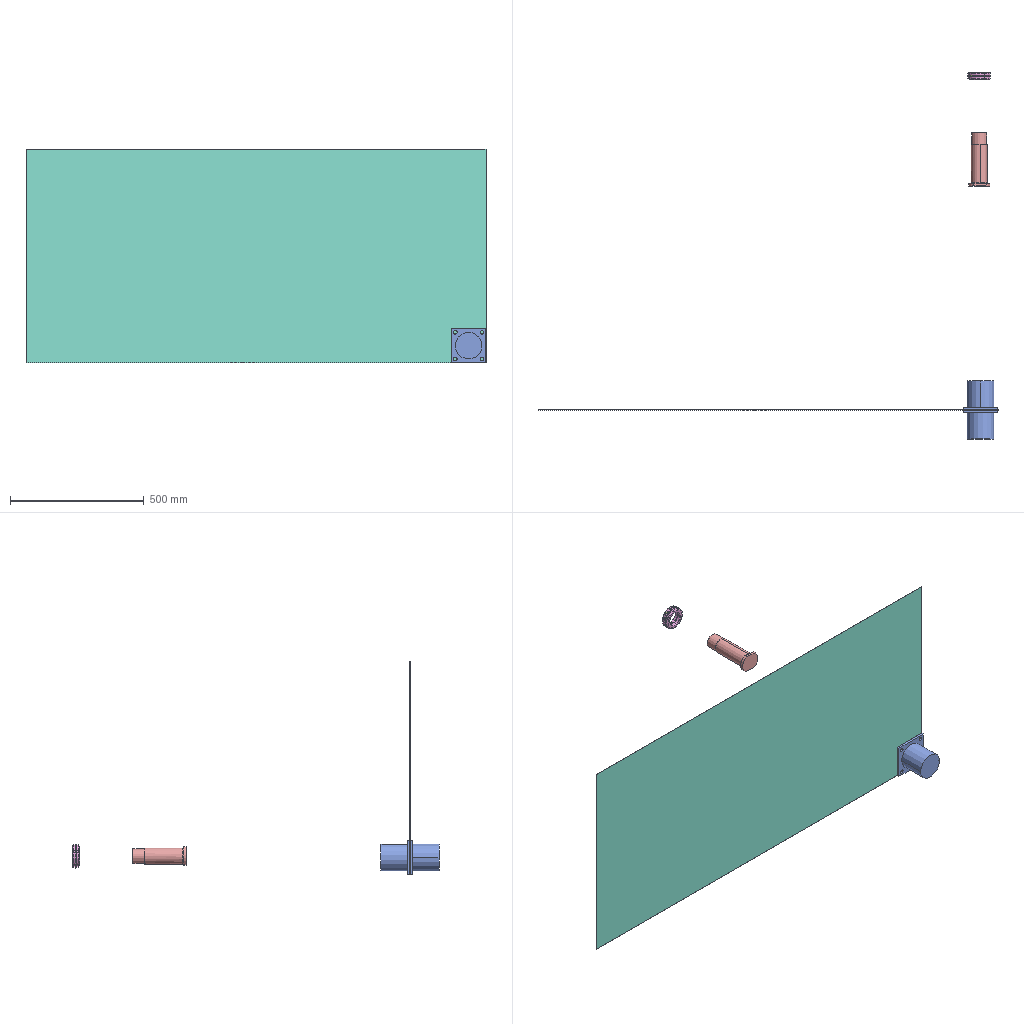Assembly | SolidWorks | 9 different items | 11 placed | box 1720 x 1369 x 800 mm
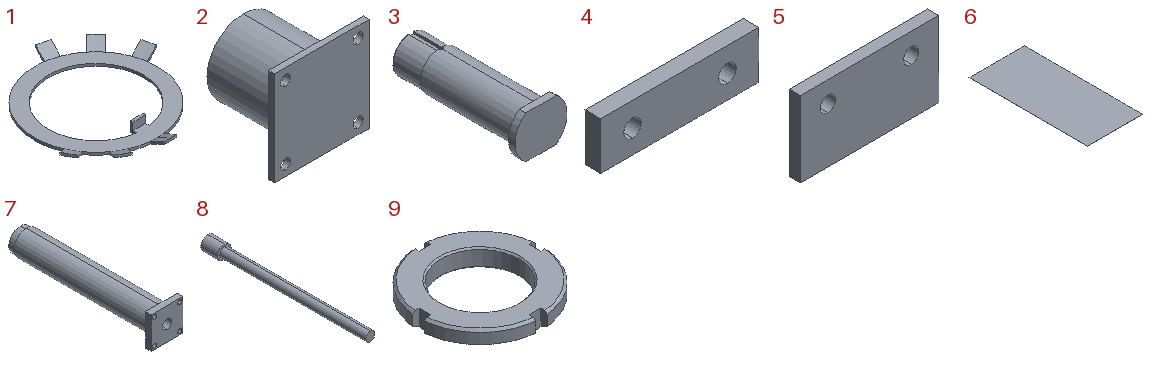Parts list (item | quantity | size | volume | features):
1 | x1 | 85.057 x 89.139 x 6 mm | 3268 mm3 | features Boss 1, Cut 1, Revolution 1
2 | x2 | 130 x 108 x 130 mm | 915672 mm3 | features Extrusion 1, HoleWzd 1, ICE 1
3 | x1 | 80 x 200 x 65 mm | 564846 mm3 | features Fillet 2, ICE 2, Chamfer 1, Revolution 1
4 | x1 | 100 x 10 x 30 mm | 28099 mm3 | features Extrusion 1, HoleWzd 1
5 | x1 | 100 x 8 x 54.5 mm | 42079 mm3 | features Extrusion 1, HoleWzd 1
6 | x1 | 800 x 1720 x 1 mm | 1376000 mm3 | features Extrusion 1
7 | x1 | 140 x 652 x 140 mm | 5526719 mm3 | features ICE 4, Extrusion 1
8 | x1 | 60 x 708 x 60 mm | 1002796 mm3 | features Revolution 1
9 | x2 | 84.623 x 84.623 x 12 mm | 36703 mm3 | features Chamfer 3, CirPattern 1, Cut 1, Extrusion 1
Mates (type | each side: item.copy, entity, surface, feature):
Concentric | 9.1 face cylinder Boss-Extrude | 9.2 face cylinder Boss-Extrude
Concentric | 1.1 face cylinder Cut-Extrude2 | 9.2 face cylinder Boss-Extrude
Coincident | 1.1 face plane Boss-Revolve | 9.2 face plane Boss-Extrude
Coincident | 9.1 face plane Boss-Extrude | 1.1 face plane Boss-Revolve
Coincident | 9.1 face plane CirPattern1 | 9.2 face plane CirPattern1
Concentric | 3.1 face cylinder Revolve1 | 9.2 face cylinder Boss-Extrude
Parallel | 3.1 face plane Cut-Extrude2 | 1.1 face plane Cut-Extrude2
Concentric | 4.1 face cylinder Ø11.0 (11) Diameter Hole1 | 5.1 face cylinder Ø11.0 (11) Diameter Hole1
Coincident | 4.1 face plane Boss-Extrude1 | 5.1 face plane Boss-Extrude1 | 2 times
Concentric | 7.1 face cylinder Cut-Extrude1 | 8.1 face cylinder Revolve1
LimitDistanceDim | 7.1 face plane Boss-Extrude1 | 8.1 face plane Revolve1
Coincident | 3.1 face plane Cut-Extrude1 | 5.1 face plane Boss-Extrude1
Coincident | 3.1 face plane Revolve1 | 5.1 face plane Boss-Extrude1
Coincident | 2.1 face plane Boss-Extrude1 | 6.1 face plane Boss-Extrude1
Concentric | 7.1 face cylinder Boss-Extrude1 | 2.2 face cylinder Ø14.0 (14) Diameter Hole1
Coincident | 7.1 face plane Boss-Extrude1 | 2.2 face plane Boss-Extrude2
Parallel | 7.1 face plane Boss-Extrude1 | 2.2 face plane Boss-Extrude1
Coincident | 2.2 face plane Boss-Extrude1 | 6.1 face plane Boss-Extrude1 | 3 times
Concentric | 2.2 face cylinder Boss-Extrude2 | 2.1 face cylinder Boss-Extrude2
Coincident | 2.2 face plane Boss-Extrude1 | 2.1 face plane Boss-Extrude1
Concentric | 3.1 face cylinder Revolve1 | 8.1 face cylinder Revolve1
Coincident | 3.1 face plane Revolve1 | 8.1 face plane Revolve1